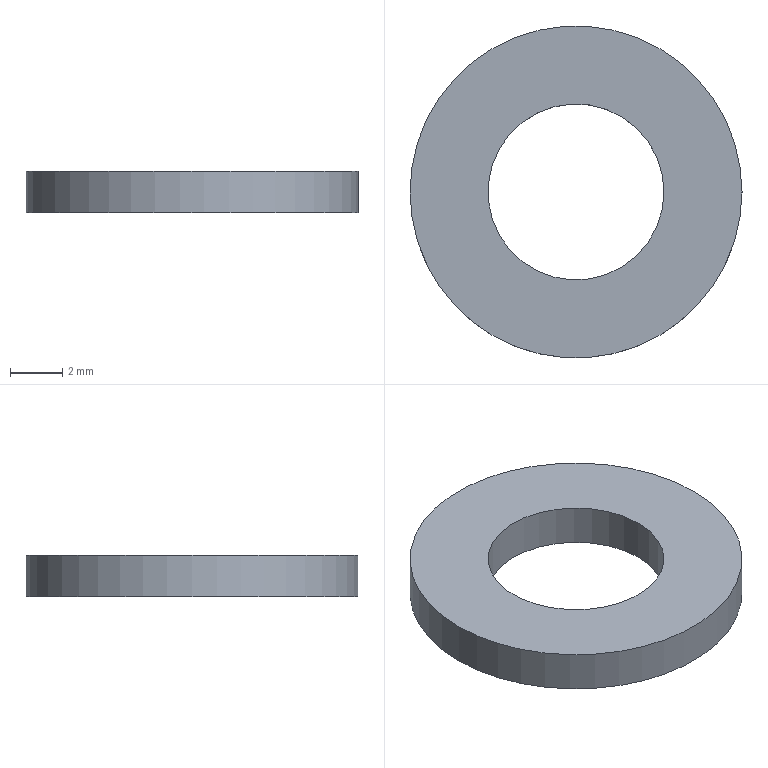Part | NX | features solid 2 | 1 solid | 4 faces | box 12.7 x 12.7 x 1.6 mm | volume 145.768 mm3 | cylinder 2 | plane 2 | commonest cylinder face diameters 6.731 x1 12.7 x1
STEP:
#1=CARTESIAN_POINT('',(6.35,0.,1.6));
#2=VERTEX_POINT('',#1);
#3=CARTESIAN_POINT('',(0.,0.,1.6));
#4=DIRECTION('',(0.,0.,-1.));
#5=DIRECTION('',(1.,0.,0.));
#6=AXIS2_PLACEMENT_3D('',#3,#4,#5);
#7=CIRCLE('',#6,6.35);
#8=EDGE_CURVE('',#2,#2,#7,.T.);
#9=ORIENTED_EDGE('',*,*,#8,.T.);
#10=EDGE_LOOP('',(#9));
#11=FACE_BOUND('',#10,.T.);
#12=CARTESIAN_POINT('',(6.35,0.,0.));
#13=VERTEX_POINT('',#12);
#14=CARTESIAN_POINT('',(0.,0.,0.));
#15=DIRECTION('',(0.,0.,-1.));
#16=DIRECTION('',(1.,0.,0.));
#17=AXIS2_PLACEMENT_3D('',#14,#15,#16);
#18=CIRCLE('',#17,6.35);
#19=EDGE_CURVE('',#13,#13,#18,.T.);
#20=ORIENTED_EDGE('',*,*,#19,.F.);
#21=EDGE_LOOP('',(#20));
#22=FACE_BOUND('',#21,.T.);
#23=CARTESIAN_POINT('',(0.,0.,1.6));
#24=DIRECTION('',(0.,0.,-1.));
#25=DIRECTION('',(-1.,0.,0.));
#26=AXIS2_PLACEMENT_3D('',#23,#24,#25);
#27=CYLINDRICAL_SURFACE('',#26,6.35);
#28=ADVANCED_FACE('',(#11,#22),#27,.T.);
#29=CARTESIAN_POINT('',(3.365,0.,1.6));
#30=VERTEX_POINT('',#29);
#31=CARTESIAN_POINT('',(0.,0.,1.6));
#32=DIRECTION('',(0.,0.,-1.));
#33=DIRECTION('',(1.,0.,0.));
#34=AXIS2_PLACEMENT_3D('',#31,#32,#33);
#35=CIRCLE('',#34,3.365);
#36=EDGE_CURVE('',#30,#30,#35,.T.);
#37=ORIENTED_EDGE('',*,*,#36,.F.);
#38=EDGE_LOOP('',(#37));
#39=FACE_BOUND('',#38,.T.);
#40=CARTESIAN_POINT('',(3.365,0.,0.));
#41=VERTEX_POINT('',#40);
#42=CARTESIAN_POINT('',(0.,0.,0.));
#43=DIRECTION('',(0.,0.,-1.));
#44=DIRECTION('',(1.,0.,0.));
#45=AXIS2_PLACEMENT_3D('',#42,#43,#44);
#46=CIRCLE('',#45,3.365);
#47=EDGE_CURVE('',#41,#41,#46,.T.);
#48=ORIENTED_EDGE('',*,*,#47,.T.);
#49=EDGE_LOOP('',(#48));
#50=FACE_BOUND('',#49,.T.);
#51=CARTESIAN_POINT('',(0.,0.,1.6));
#52=DIRECTION('',(0.,0.,-1.));
#53=DIRECTION('',(-1.,0.,0.));
#54=AXIS2_PLACEMENT_3D('',#51,#52,#53);
#55=CYLINDRICAL_SURFACE('',#54,3.365);
#56=ADVANCED_FACE('',(#39,#50),#55,.F.);
#57=ORIENTED_EDGE('',*,*,#8,.F.);
#58=EDGE_LOOP('',(#57));
#59=FACE_BOUND('',#58,.T.);
#60=ORIENTED_EDGE('',*,*,#36,.T.);
#61=EDGE_LOOP('',(#60));
#62=FACE_BOUND('',#61,.T.);
#63=CARTESIAN_POINT('',(0.,0.,1.6));
#64=DIRECTION('',(0.,0.,-1.));
#65=DIRECTION('',(-1.,0.,0.));
#66=AXIS2_PLACEMENT_3D('',#63,#64,#65);
#67=PLANE('',#66);
#68=ADVANCED_FACE('',(#59,#62),#67,.F.);
#69=ORIENTED_EDGE('',*,*,#19,.T.);
#70=EDGE_LOOP('',(#69));
#71=FACE_BOUND('',#70,.T.);
#72=ORIENTED_EDGE('',*,*,#47,.F.);
#73=EDGE_LOOP('',(#72));
#74=FACE_BOUND('',#73,.T.);
#75=CARTESIAN_POINT('',(0.,0.,0.));
#76=DIRECTION('',(0.,0.,-1.));
#77=DIRECTION('',(-1.,0.,0.));
#78=AXIS2_PLACEMENT_3D('',#75,#76,#77);
#79=PLANE('',#78);
#80=ADVANCED_FACE('',(#71,#74),#79,.T.);
#81=CLOSED_SHELL('',(#28,#56,#68,#80));
#82=MANIFOLD_SOLID_BREP('',#81);
#83=(LENGTH_UNIT()NAMED_UNIT(*)SI_UNIT(.MILLI.,.METRE.));
#84=UNCERTAINTY_MEASURE_WITH_UNIT(LENGTH_MEASURE(0.00001),#83,'','');
#85=(NAMED_UNIT(*)PLANE_ANGLE_UNIT()SI_UNIT($,.RADIAN.));
#86=(NAMED_UNIT(*)SI_UNIT($,.STERADIAN.)SOLID_ANGLE_UNIT());
#87=(GEOMETRIC_REPRESENTATION_CONTEXT(3)GLOBAL_UNCERTAINTY_ASSIGNED_CONTEXT((#84))GLOBAL_UNIT_ASSIGNED_CONTEXT((#83,#85,#86))REPRESENTATION_CONTEXT('',''));
#88=ADVANCED_BREP_SHAPE_REPRESENTATION('',(#82),#87);